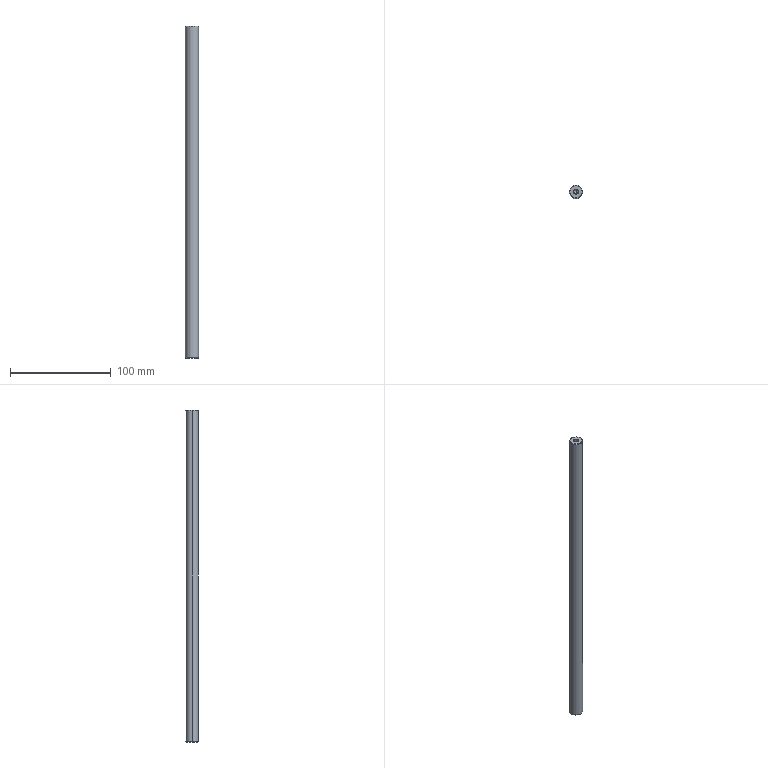Part | STEP file | 001-003-SCD21_D13_L330_M5 | 1 solid | 14 faces | box 13 x 13 x 330 mm | volume 43651 mm3 | cone 8 | cylinder 4 | plane 2 | commonest cylinder face diameters 4.134 x2 13 x2
STEP:
#1=CARTESIAN_POINT('',(0.,0.,0.));
#2=DIRECTION('',(0.,0.,1.));
#3=DIRECTION('',(1.,0.,0.));
#4=AXIS2_PLACEMENT_3D('',#1,#2,#3);
#5=CARTESIAN_POINT('',(0.,2.067,-10.));
#6=VERTEX_POINT('',#5);
#7=CARTESIAN_POINT('',(0.,-2.067,-10.));
#8=VERTEX_POINT('',#7);
#9=CARTESIAN_POINT('',(0.,0.,-10.));
#10=DIRECTION('',(0.,0.,1.));
#11=DIRECTION('',(0.,-1.,0.));
#12=AXIS2_PLACEMENT_3D('',#9,#10,#11);
#13=CIRCLE('',#12,2.067);
#14=CARTESIAN_POINT('',(0.,0.,988.807));
#15=DIRECTION('',(0.,0.,1.));
#16=DIRECTION('',(0.,-1.,0.));
#17=AXIS2_PLACEMENT_3D('',#14,#15,#16);
#18=CONICAL_SURFACE('',#17,1732.051,1.047);
#19=CARTESIAN_POINT('',(0.,-998.807));
#20=DIRECTION('',(1.,0.));
#21=VECTOR('',#20,1.);
#22=LINE('',#19,#21);
#23=(GEOMETRIC_REPRESENTATION_CONTEXT(2)PARAMETRIC_REPRESENTATION_CONTEXT()REPRESENTATION_CONTEXT('',''));
#24=DEFINITIONAL_REPRESENTATION('',(#22),#23);
#25=PCURVE('',#18,#24);
#26=CARTESIAN_POINT('',(0.,0.,-11.193));
#27=DIRECTION('',(0.,0.,1.));
#28=DIRECTION('',(0.,-1.,0.));
#29=AXIS2_PLACEMENT_3D('',#26,#27,#28);
#30=CYLINDRICAL_SURFACE('',#29,2.067);
#31=CARTESIAN_POINT('',(0.,1.193));
#32=DIRECTION('',(1.,0.));
#33=VECTOR('',#32,1.);
#34=LINE('',#31,#33);
#35=(GEOMETRIC_REPRESENTATION_CONTEXT(2)PARAMETRIC_REPRESENTATION_CONTEXT()REPRESENTATION_CONTEXT('',''));
#36=DEFINITIONAL_REPRESENTATION('',(#34),#35);
#37=PCURVE('',#30,#36);
#38=SURFACE_CURVE('',#13,(#25,#37),.PCURVE_S1.);
#39=EDGE_CURVE('',#6,#8,#38,.T.);
#40=ORIENTED_EDGE('',*,*,#39,.F.);
#41=CARTESIAN_POINT('',(0.,0.,-11.193));
#42=VERTEX_POINT('',#41);
#43=CARTESIAN_POINT('',(0.,0.,-11.193));
#44=DIRECTION('',(0.,0.866,0.5));
#45=VECTOR('',#44,1.);
#46=LINE('',#43,#45);
#47=CARTESIAN_POINT('',(3.142,-1000.));
#48=CARTESIAN_POINT('',(3.142,-999.982));
#49=CARTESIAN_POINT('',(3.142,-999.946));
#50=CARTESIAN_POINT('',(3.142,-999.892));
#51=CARTESIAN_POINT('',(3.142,-999.837));
#52=CARTESIAN_POINT('',(3.142,-999.783));
#53=CARTESIAN_POINT('',(3.142,-999.729));
#54=CARTESIAN_POINT('',(3.142,-999.675));
#55=CARTESIAN_POINT('',(3.142,-999.62));
#56=CARTESIAN_POINT('',(3.142,-999.566));
#57=CARTESIAN_POINT('',(3.142,-999.512));
#58=CARTESIAN_POINT('',(3.142,-999.458));
#59=CARTESIAN_POINT('',(3.142,-999.403));
#60=CARTESIAN_POINT('',(3.142,-999.349));
#61=CARTESIAN_POINT('',(3.142,-999.295));
#62=CARTESIAN_POINT('',(3.142,-999.241));
#63=CARTESIAN_POINT('',(3.142,-999.186));
#64=CARTESIAN_POINT('',(3.142,-999.132));
#65=CARTESIAN_POINT('',(3.142,-999.078));
#66=CARTESIAN_POINT('',(3.142,-999.024));
#67=CARTESIAN_POINT('',(3.142,-998.969));
#68=CARTESIAN_POINT('',(3.142,-998.915));
#69=CARTESIAN_POINT('',(3.142,-998.861));
#70=CARTESIAN_POINT('',(3.142,-998.825));
#71=CARTESIAN_POINT('',(3.142,-998.807));
#72=B_SPLINE_CURVE_WITH_KNOTS('',3,(#47,#48,#49,#50,#51,#52,#53,#54,#55,#56,#57,#58,#59,#60,#61,#62,#63,#64,#65,#66,#67,#68,#69,#70,#71),.UNSPECIFIED.,.F.,.F.,(4,1,1,1,1,1,1,1,1,1,1,1,1,1,1,1,1,1,1,1,1,1,4),(0.,0.1085,0.217,0.3255,0.434,0.5424,0.6509,0.7594,0.8679,0.9764,1.085,1.193,1.302,1.41,1.519,1.627,1.736,1.844,1.953,2.061,2.17,2.278,2.387),.QUASI_UNIFORM_KNOTS.);
#73=(GEOMETRIC_REPRESENTATION_CONTEXT(2)PARAMETRIC_REPRESENTATION_CONTEXT()REPRESENTATION_CONTEXT('',''));
#74=DEFINITIONAL_REPRESENTATION('',(#72),#73);
#75=PCURVE('',#18,#74);
#76=CARTESIAN_POINT('',(0.,0.,988.807));
#77=DIRECTION('',(0.,0.,1.));
#78=DIRECTION('',(0.,-1.,0.));
#79=AXIS2_PLACEMENT_3D('',#76,#77,#78);
#80=CONICAL_SURFACE('',#79,1732.051,1.047);
#81=CARTESIAN_POINT('',(3.142,-1000.));
#82=CARTESIAN_POINT('',(3.142,-999.982));
#83=CARTESIAN_POINT('',(3.142,-999.946));
#84=CARTESIAN_POINT('',(3.142,-999.892));
#85=CARTESIAN_POINT('',(3.142,-999.837));
#86=CARTESIAN_POINT('',(3.142,-999.783));
#87=CARTESIAN_POINT('',(3.142,-999.729));
#88=CARTESIAN_POINT('',(3.142,-999.675));
#89=CARTESIAN_POINT('',(3.142,-999.62));
#90=CARTESIAN_POINT('',(3.142,-999.566));
#91=CARTESIAN_POINT('',(3.142,-999.512));
#92=CARTESIAN_POINT('',(3.142,-999.458));
#93=CARTESIAN_POINT('',(3.142,-999.403));
#94=CARTESIAN_POINT('',(3.142,-999.349));
#95=CARTESIAN_POINT('',(3.142,-999.295));
#96=CARTESIAN_POINT('',(3.142,-999.241));
#97=CARTESIAN_POINT('',(3.142,-999.186));
#98=CARTESIAN_POINT('',(3.142,-999.132));
#99=CARTESIAN_POINT('',(3.142,-999.078));
#100=CARTESIAN_POINT('',(3.142,-999.024));
#101=CARTESIAN_POINT('',(3.142,-998.969));
#102=CARTESIAN_POINT('',(3.142,-998.915));
#103=CARTESIAN_POINT('',(3.142,-998.861));
#104=CARTESIAN_POINT('',(3.142,-998.825));
#105=CARTESIAN_POINT('',(3.142,-998.807));
#106=B_SPLINE_CURVE_WITH_KNOTS('',3,(#81,#82,#83,#84,#85,#86,#87,#88,#89,#90,#91,#92,#93,#94,#95,#96,#97,#98,#99,#100,#101,#102,#103,#104,#105),.UNSPECIFIED.,.F.,.F.,(4,1,1,1,1,1,1,1,1,1,1,1,1,1,1,1,1,1,1,1,1,1,4),(0.,0.1085,0.217,0.3255,0.434,0.5424,0.6509,0.7594,0.8679,0.9764,1.085,1.193,1.302,1.41,1.519,1.627,1.736,1.844,1.953,2.061,2.17,2.278,2.387),.QUASI_UNIFORM_KNOTS.);
#107=(GEOMETRIC_REPRESENTATION_CONTEXT(2)PARAMETRIC_REPRESENTATION_CONTEXT()REPRESENTATION_CONTEXT('',''));
#108=DEFINITIONAL_REPRESENTATION('',(#106),#107);
#109=PCURVE('',#80,#108);
#110=SURFACE_CURVE('',#46,(#75,#109),.PCURVE_S1.);
#111=EDGE_CURVE('',#42,#6,#110,.T.);
#112=ORIENTED_EDGE('',*,*,#111,.F.);
#113=CARTESIAN_POINT('',(0.,0.,-11.193));
#114=DIRECTION('',(0.,-0.866,0.5));
#115=VECTOR('',#114,1.);
#116=LINE('',#113,#115);
#117=CARTESIAN_POINT('',(6.283,-1000.));
#118=DIRECTION('',(0.,1.));
#119=VECTOR('',#118,1.);
#120=LINE('',#117,#119);
#121=(GEOMETRIC_REPRESENTATION_CONTEXT(2)PARAMETRIC_REPRESENTATION_CONTEXT()REPRESENTATION_CONTEXT('',''));
#122=DEFINITIONAL_REPRESENTATION('',(#120),#121);
#123=PCURVE('',#18,#122);
#124=CARTESIAN_POINT('',(0.,-1000.));
#125=DIRECTION('',(0.,1.));
#126=VECTOR('',#125,1.);
#127=LINE('',#124,#126);
#128=(GEOMETRIC_REPRESENTATION_CONTEXT(2)PARAMETRIC_REPRESENTATION_CONTEXT()REPRESENTATION_CONTEXT('',''));
#129=DEFINITIONAL_REPRESENTATION('',(#127),#128);
#130=PCURVE('',#80,#129);
#131=SURFACE_CURVE('',#116,(#123,#130),.PCURVE_S1.);
#132=EDGE_CURVE('',#42,#8,#131,.T.);
#133=ORIENTED_EDGE('',*,*,#132,.T.);
#134=EDGE_LOOP('',(#40,#112,#133));
#135=FACE_BOUND('',#134,.F.);
#136=ADVANCED_FACE('',(#135),#18,.F.);
#137=CARTESIAN_POINT('',(0.,-2.067,-0.433));
#138=VERTEX_POINT('',#137);
#139=CARTESIAN_POINT('',(0.,-2.067,-11.193));
#140=DIRECTION('',(0.,0.,1.));
#141=VECTOR('',#140,1.);
#142=LINE('',#139,#141);
#143=CARTESIAN_POINT('',(6.283,0.));
#144=DIRECTION('',(0.,1.));
#145=VECTOR('',#144,1.);
#146=LINE('',#143,#145);
#147=(GEOMETRIC_REPRESENTATION_CONTEXT(2)PARAMETRIC_REPRESENTATION_CONTEXT()REPRESENTATION_CONTEXT('',''));
#148=DEFINITIONAL_REPRESENTATION('',(#146),#147);
#149=PCURVE('',#30,#148);
#150=CARTESIAN_POINT('',(0.,0.,-11.193));
#151=DIRECTION('',(0.,0.,1.));
#152=DIRECTION('',(0.,-1.,0.));
#153=AXIS2_PLACEMENT_3D('',#150,#151,#152);
#154=CYLINDRICAL_SURFACE('',#153,2.067);
#155=CARTESIAN_POINT('',(0.,0.));
#156=DIRECTION('',(0.,1.));
#157=VECTOR('',#156,1.);
#158=LINE('',#155,#157);
#159=(GEOMETRIC_REPRESENTATION_CONTEXT(2)PARAMETRIC_REPRESENTATION_CONTEXT()REPRESENTATION_CONTEXT('',''));
#160=DEFINITIONAL_REPRESENTATION('',(#158),#159);
#161=PCURVE('',#154,#160);
#162=SURFACE_CURVE('',#142,(#149,#161),.PCURVE_S1.);
#163=EDGE_CURVE('',#8,#138,#162,.T.);
#164=ORIENTED_EDGE('',*,*,#163,.T.);
#165=CARTESIAN_POINT('',(0.,2.067,-0.433));
#166=VERTEX_POINT('',#165);
#167=CARTESIAN_POINT('',(0.,0.,-0.433));
#168=DIRECTION('',(0.,0.,1.));
#169=DIRECTION('',(0.,-1.,0.));
#170=AXIS2_PLACEMENT_3D('',#167,#168,#169);
#171=CIRCLE('',#170,2.067);
#172=CARTESIAN_POINT('',(0.,10.76));
#173=DIRECTION('',(1.,0.));
#174=VECTOR('',#173,1.);
#175=LINE('',#172,#174);
#176=(GEOMETRIC_REPRESENTATION_CONTEXT(2)PARAMETRIC_REPRESENTATION_CONTEXT()REPRESENTATION_CONTEXT('',''));
#177=DEFINITIONAL_REPRESENTATION('',(#175),#176);
#178=PCURVE('',#30,#177);
#179=CARTESIAN_POINT('',(0.,0.,-0.433));
#180=DIRECTION('',(0.,0.,1.));
#181=DIRECTION('',(0.,-1.,0.));
#182=AXIS2_PLACEMENT_3D('',#179,#180,#181);
#183=CONICAL_SURFACE('',#182,2.067,0.7854);
#184=CARTESIAN_POINT('',(0.,0.));
#185=DIRECTION('',(1.,0.));
#186=VECTOR('',#185,1.);
#187=LINE('',#184,#186);
#188=(GEOMETRIC_REPRESENTATION_CONTEXT(2)PARAMETRIC_REPRESENTATION_CONTEXT()REPRESENTATION_CONTEXT('',''));
#189=DEFINITIONAL_REPRESENTATION('',(#187),#188);
#190=PCURVE('',#183,#189);
#191=SURFACE_CURVE('',#171,(#178,#190),.PCURVE_S1.);
#192=EDGE_CURVE('',#166,#138,#191,.T.);
#193=ORIENTED_EDGE('',*,*,#192,.F.);
#194=CARTESIAN_POINT('',(0.,2.067,-11.193));
#195=DIRECTION('',(0.,0.,1.));
#196=VECTOR('',#195,1.);
#197=LINE('',#194,#196);
#198=CARTESIAN_POINT('',(3.142,0.));
#199=DIRECTION('',(0.,1.));
#200=VECTOR('',#199,1.);
#201=LINE('',#198,#200);
#202=(GEOMETRIC_REPRESENTATION_CONTEXT(2)PARAMETRIC_REPRESENTATION_CONTEXT()REPRESENTATION_CONTEXT('',''));
#203=DEFINITIONAL_REPRESENTATION('',(#201),#202);
#204=PCURVE('',#30,#203);
#205=CARTESIAN_POINT('',(3.142,0.));
#206=DIRECTION('',(0.,1.));
#207=VECTOR('',#206,1.);
#208=LINE('',#205,#207);
#209=(GEOMETRIC_REPRESENTATION_CONTEXT(2)PARAMETRIC_REPRESENTATION_CONTEXT()REPRESENTATION_CONTEXT('',''));
#210=DEFINITIONAL_REPRESENTATION('',(#208),#209);
#211=PCURVE('',#154,#210);
#212=SURFACE_CURVE('',#197,(#204,#211),.PCURVE_S1.);
#213=EDGE_CURVE('',#6,#166,#212,.T.);
#214=ORIENTED_EDGE('',*,*,#213,.F.);
#215=ORIENTED_EDGE('',*,*,#39,.T.);
#216=EDGE_LOOP('',(#164,#193,#214,#215));
#217=FACE_BOUND('',#216,.F.);
#218=ADVANCED_FACE('',(#217),#30,.F.);
#219=CARTESIAN_POINT('',(0.,-2.5,0.));
#220=VERTEX_POINT('',#219);
#221=CARTESIAN_POINT('',(0.,-2.067,-0.433));
#222=DIRECTION('',(0.,-0.7071,0.7071));
#223=VECTOR('',#222,1.);
#224=LINE('',#221,#223);
#225=CARTESIAN_POINT('',(6.283,0.));
#226=DIRECTION('',(0.,1.));
#227=VECTOR('',#226,1.);
#228=LINE('',#225,#227);
#229=(GEOMETRIC_REPRESENTATION_CONTEXT(2)PARAMETRIC_REPRESENTATION_CONTEXT()REPRESENTATION_CONTEXT('',''));
#230=DEFINITIONAL_REPRESENTATION('',(#228),#229);
#231=PCURVE('',#183,#230);
#232=CARTESIAN_POINT('',(0.,0.,-0.433));
#233=DIRECTION('',(0.,0.,1.));
#234=DIRECTION('',(0.,-1.,0.));
#235=AXIS2_PLACEMENT_3D('',#232,#233,#234);
#236=CONICAL_SURFACE('',#235,2.067,0.7854);
#237=CARTESIAN_POINT('',(0.,0.));
#238=DIRECTION('',(0.,1.));
#239=VECTOR('',#238,1.);
#240=LINE('',#237,#239);
#241=(GEOMETRIC_REPRESENTATION_CONTEXT(2)PARAMETRIC_REPRESENTATION_CONTEXT()REPRESENTATION_CONTEXT('',''));
#242=DEFINITIONAL_REPRESENTATION('',(#240),#241);
#243=PCURVE('',#236,#242);
#244=SURFACE_CURVE('',#224,(#231,#243),.PCURVE_S1.);
#245=EDGE_CURVE('',#138,#220,#244,.T.);
#246=ORIENTED_EDGE('',*,*,#245,.T.);
#247=CARTESIAN_POINT('',(0.,2.5,0.));
#248=VERTEX_POINT('',#247);
#249=CARTESIAN_POINT('',(0.,0.,0.));
#250=DIRECTION('',(0.,0.,1.));
#251=DIRECTION('',(0.,-1.,0.));
#252=AXIS2_PLACEMENT_3D('',#249,#250,#251);
#253=CIRCLE('',#252,2.5);
#254=CARTESIAN_POINT('',(0.,0.433));
#255=DIRECTION('',(1.,0.));
#256=VECTOR('',#255,1.);
#257=LINE('',#254,#256);
#258=(GEOMETRIC_REPRESENTATION_CONTEXT(2)PARAMETRIC_REPRESENTATION_CONTEXT()REPRESENTATION_CONTEXT('',''));
#259=DEFINITIONAL_REPRESENTATION('',(#257),#258);
#260=PCURVE('',#183,#259);
#261=CARTESIAN_POINT('',(0.,0.,0.));
#262=DIRECTION('',(0.,0.,-1.));
#263=DIRECTION('',(-1.,0.,0.));
#264=AXIS2_PLACEMENT_3D('',#261,#262,#263);
#265=PLANE('',#264);
#266=CARTESIAN_POINT('',(0.,-2.5));
#267=CARTESIAN_POINT('',(-4.33,-2.5));
#268=CARTESIAN_POINT('',(-2.165,1.25));
#269=CARTESIAN_POINT('',(0.,5.));
#270=CARTESIAN_POINT('',(2.165,1.25));
#271=CARTESIAN_POINT('',(4.33,-2.5));
#272=CARTESIAN_POINT('',(0.,-2.5));
#273=(BOUNDED_CURVE()B_SPLINE_CURVE(2,(#266,#267,#268,#269,#270,#271,#272),.UNSPECIFIED.,.T.,.F.)B_SPLINE_CURVE_WITH_KNOTS((1,2,2,2,2,1),(-2.094,0.,2.094,4.189,6.283,8.378),.UNSPECIFIED.)CURVE()GEOMETRIC_REPRESENTATION_ITEM()RATIONAL_B_SPLINE_CURVE((1.,0.5,1.,0.5,1.,0.5,1.))REPRESENTATION_ITEM(''));
#274=(GEOMETRIC_REPRESENTATION_CONTEXT(2)PARAMETRIC_REPRESENTATION_CONTEXT()REPRESENTATION_CONTEXT('',''));
#275=DEFINITIONAL_REPRESENTATION('',(#273),#274);
#276=PCURVE('',#265,#275);
#277=SURFACE_CURVE('',#253,(#260,#276),.PCURVE_S1.);
#278=EDGE_CURVE('',#248,#220,#277,.T.);
#279=ORIENTED_EDGE('',*,*,#278,.F.);
#280=CARTESIAN_POINT('',(0.,2.067,-0.433));
#281=DIRECTION('',(0.,0.7071,0.7071));
#282=VECTOR('',#281,1.);
#283=LINE('',#280,#282);
#284=CARTESIAN_POINT('',(3.142,0.));
#285=DIRECTION('',(0.,1.));
#286=VECTOR('',#285,1.);
#287=LINE('',#284,#286);
#288=(GEOMETRIC_REPRESENTATION_CONTEXT(2)PARAMETRIC_REPRESENTATION_CONTEXT()REPRESENTATION_CONTEXT('',''));
#289=DEFINITIONAL_REPRESENTATION('',(#287),#288);
#290=PCURVE('',#183,#289);
#291=CARTESIAN_POINT('',(3.142,0.));
#292=DIRECTION('',(0.,1.));
#293=VECTOR('',#292,1.);
#294=LINE('',#291,#293);
#295=(GEOMETRIC_REPRESENTATION_CONTEXT(2)PARAMETRIC_REPRESENTATION_CONTEXT()REPRESENTATION_CONTEXT('',''));
#296=DEFINITIONAL_REPRESENTATION('',(#294),#295);
#297=PCURVE('',#236,#296);
#298=SURFACE_CURVE('',#283,(#290,#297),.PCURVE_S1.);
#299=EDGE_CURVE('',#166,#248,#298,.T.);
#300=ORIENTED_EDGE('',*,*,#299,.F.);
#301=ORIENTED_EDGE('',*,*,#192,.T.);
#302=EDGE_LOOP('',(#246,#279,#300,#301));
#303=FACE_BOUND('',#302,.F.);
#304=ADVANCED_FACE('',(#303),#183,.F.);
#305=CARTESIAN_POINT('',(6.,0.,-330.));
#306=VERTEX_POINT('',#305);
#307=CARTESIAN_POINT('',(-6.,0.,-330.));
#308=VERTEX_POINT('',#307);
#309=CARTESIAN_POINT('',(0.,0.,-330.));
#310=DIRECTION('',(0.,0.,1.));
#311=DIRECTION('',(1.,0.,0.));
#312=AXIS2_PLACEMENT_3D('',#309,#310,#311);
#313=CIRCLE('',#312,6.);
#314=CARTESIAN_POINT('',(0.,0.,-330.));
#315=DIRECTION('',(0.,0.,1.));
#316=DIRECTION('',(1.,0.,0.));
#317=AXIS2_PLACEMENT_3D('',#314,#315,#316);
#318=CONICAL_SURFACE('',#317,6.,0.7854);
#319=CARTESIAN_POINT('',(0.,0.));
#320=DIRECTION('',(1.,0.));
#321=VECTOR('',#320,1.);
#322=LINE('',#319,#321);
#323=(GEOMETRIC_REPRESENTATION_CONTEXT(2)PARAMETRIC_REPRESENTATION_CONTEXT()REPRESENTATION_CONTEXT('',''));
#324=DEFINITIONAL_REPRESENTATION('',(#322),#323);
#325=PCURVE('',#318,#324);
#326=CARTESIAN_POINT('',(0.,6.,-330.));
#327=DIRECTION('',(0.,0.,1.));
#328=DIRECTION('',(1.,0.,0.));
#329=AXIS2_PLACEMENT_3D('',#326,#327,#328);
#330=PLANE('',#329);
#331=CARTESIAN_POINT('',(0.,-6.));
#332=DIRECTION('',(1.,0.));
#333=AXIS2_PLACEMENT_2D('',#331,#332);
#334=CIRCLE('',#333,6.);
#335=(GEOMETRIC_REPRESENTATION_CONTEXT(2)PARAMETRIC_REPRESENTATION_CONTEXT()REPRESENTATION_CONTEXT('',''));
#336=DEFINITIONAL_REPRESENTATION('',(#334),#335);
#337=PCURVE('',#330,#336);
#338=SURFACE_CURVE('',#313,(#325,#337),.PCURVE_S1.);
#339=EDGE_CURVE('',#306,#308,#338,.T.);
#340=ORIENTED_EDGE('',*,*,#339,.T.);
#341=CARTESIAN_POINT('',(-6.5,0.,-329.5));
#342=VERTEX_POINT('',#341);
#343=CARTESIAN_POINT('',(-6.,0.,-330.));
#344=DIRECTION('',(-0.7071,0.,0.7071));
#345=VECTOR('',#344,1.);
#346=LINE('',#343,#345);
#347=CARTESIAN_POINT('',(3.142,0.));
#348=DIRECTION('',(0.,1.));
#349=VECTOR('',#348,1.);
#350=LINE('',#347,#349);
#351=(GEOMETRIC_REPRESENTATION_CONTEXT(2)PARAMETRIC_REPRESENTATION_CONTEXT()REPRESENTATION_CONTEXT('',''));
#352=DEFINITIONAL_REPRESENTATION('',(#350),#351);
#353=PCURVE('',#318,#352);
#354=CARTESIAN_POINT('',(0.,0.,-330.));
#355=DIRECTION('',(0.,0.,1.));
#356=DIRECTION('',(1.,0.,0.));
#357=AXIS2_PLACEMENT_3D('',#354,#355,#356);
#358=CONICAL_SURFACE('',#357,6.,0.7854);
#359=CARTESIAN_POINT('',(3.142,0.));
#360=DIRECTION('',(0.,1.));
#361=VECTOR('',#360,1.);
#362=LINE('',#359,#361);
#363=(GEOMETRIC_REPRESENTATION_CONTEXT(2)PARAMETRIC_REPRESENTATION_CONTEXT()REPRESENTATION_CONTEXT('',''));
#364=DEFINITIONAL_REPRESENTATION('',(#362),#363);
#365=PCURVE('',#358,#364);
#366=SURFACE_CURVE('',#346,(#353,#365),.PCURVE_S1.);
#367=EDGE_CURVE('',#308,#342,#366,.T.);
#368=ORIENTED_EDGE('',*,*,#367,.T.);
#369=CARTESIAN_POINT('',(6.5,0.,-329.5));
#370=VERTEX_POINT('',#369);
#371=CARTESIAN_POINT('',(0.,0.,-329.5));
#372=DIRECTION('',(0.,0.,1.));
#373=DIRECTION('',(1.,0.,0.));
#374=AXIS2_PLACEMENT_3D('',#371,#372,#373);
#375=CIRCLE('',#374,6.5);
#376=CARTESIAN_POINT('',(0.,0.5));
#377=DIRECTION('',(1.,0.));
#378=VECTOR('',#377,1.);
#379=LINE('',#376,#378);
#380=(GEOMETRIC_REPRESENTATION_CONTEXT(2)PARAMETRIC_REPRESENTATION_CONTEXT()REPRESENTATION_CONTEXT('',''));
#381=DEFINITIONAL_REPRESENTATION('',(#379),#380);
#382=PCURVE('',#318,#381);
#383=CARTESIAN_POINT('',(0.,0.,-330.));
#384=DIRECTION('',(0.,0.,1.));
#385=DIRECTION('',(1.,0.,0.));
#386=AXIS2_PLACEMENT_3D('',#383,#384,#385);
#387=CYLINDRICAL_SURFACE('',#386,6.5);
#388=CARTESIAN_POINT('',(0.,0.5));
#389=DIRECTION('',(1.,0.));
#390=VECTOR('',#389,1.);
#391=LINE('',#388,#390);
#392=(GEOMETRIC_REPRESENTATION_CONTEXT(2)PARAMETRIC_REPRESENTATION_CONTEXT()REPRESENTATION_CONTEXT('',''));
#393=DEFINITIONAL_REPRESENTATION('',(#391),#392);
#394=PCURVE('',#387,#393);
#395=SURFACE_CURVE('',#375,(#382,#394),.PCURVE_S1.);
#396=EDGE_CURVE('',#370,#342,#395,.T.);
#397=ORIENTED_EDGE('',*,*,#396,.F.);
#398=CARTESIAN_POINT('',(6.,0.,-330.));
#399=DIRECTION('',(0.7071,0.,0.7071));
#400=VECTOR('',#399,1.);
#401=LINE('',#398,#400);
#402=CARTESIAN_POINT('',(0.,0.));
#403=DIRECTION('',(0.,1.));
#404=VECTOR('',#403,1.);
#405=LINE('',#402,#404);
#406=(GEOMETRIC_REPRESENTATION_CONTEXT(2)PARAMETRIC_REPRESENTATION_CONTEXT()REPRESENTATION_CONTEXT('',''));
#407=DEFINITIONAL_REPRESENTATION('',(#405),#406);
#408=PCURVE('',#318,#407);
#409=CARTESIAN_POINT('',(6.283,0.));
#410=DIRECTION('',(0.,1.));
#411=VECTOR('',#410,1.);
#412=LINE('',#409,#411);
#413=(GEOMETRIC_REPRESENTATION_CONTEXT(2)PARAMETRIC_REPRESENTATION_CONTEXT()REPRESENTATION_CONTEXT('',''));
#414=DEFINITIONAL_REPRESENTATION('',(#412),#413);
#415=PCURVE('',#358,#414);
#416=SURFACE_CURVE('',#401,(#408,#415),.PCURVE_S1.);
#417=EDGE_CURVE('',#306,#370,#416,.T.);
#418=ORIENTED_EDGE('',*,*,#417,.F.);
#419=EDGE_LOOP('',(#340,#368,#397,#418));
#420=FACE_BOUND('',#419,.T.);
#421=ADVANCED_FACE('',(#420),#318,.T.);
#422=ORIENTED_EDGE('',*,*,#396,.T.);
#423=CARTESIAN_POINT('',(-6.5,0.,-0.5));
#424=VERTEX_POINT('',#423);
#425=CARTESIAN_POINT('',(-6.5,0.,-330.));
#426=DIRECTION('',(0.,0.,1.));
#427=VECTOR('',#426,1.);
#428=LINE('',#425,#427);
#429=CARTESIAN_POINT('',(3.142,0.));
#430=DIRECTION('',(0.,1.));
#431=VECTOR('',#430,1.);
#432=LINE('',#429,#431);
#433=(GEOMETRIC_REPRESENTATION_CONTEXT(2)PARAMETRIC_REPRESENTATION_CONTEXT()REPRESENTATION_CONTEXT('',''));
#434=DEFINITIONAL_REPRESENTATION('',(#432),#433);
#435=PCURVE('',#387,#434);
#436=CARTESIAN_POINT('',(0.,0.,-330.));
#437=DIRECTION('',(0.,0.,1.));
#438=DIRECTION('',(1.,0.,0.));
#439=AXIS2_PLACEMENT_3D('',#436,#437,#438);
#440=CYLINDRICAL_SURFACE('',#439,6.5);
#441=CARTESIAN_POINT('',(3.142,0.));
#442=DIRECTION('',(0.,1.));
#443=VECTOR('',#442,1.);
#444=LINE('',#441,#443);
#445=(GEOMETRIC_REPRESENTATION_CONTEXT(2)PARAMETRIC_REPRESENTATION_CONTEXT()REPRESENTATION_CONTEXT('',''));
#446=DEFINITIONAL_REPRESENTATION('',(#444),#445);
#447=PCURVE('',#440,#446);
#448=SURFACE_CURVE('',#428,(#435,#447),.PCURVE_S1.);
#449=EDGE_CURVE('',#342,#424,#448,.T.);
#450=ORIENTED_EDGE('',*,*,#449,.T.);
#451=CARTESIAN_POINT('',(6.5,0.,-0.5));
#452=VERTEX_POINT('',#451);
#453=CARTESIAN_POINT('',(0.,0.,-0.5));
#454=DIRECTION('',(0.,0.,1.));
#455=DIRECTION('',(1.,0.,0.));
#456=AXIS2_PLACEMENT_3D('',#453,#454,#455);
#457=CIRCLE('',#456,6.5);
#458=CARTESIAN_POINT('',(0.,329.5));
#459=DIRECTION('',(1.,0.));
#460=VECTOR('',#459,1.);
#461=LINE('',#458,#460);
#462=(GEOMETRIC_REPRESENTATION_CONTEXT(2)PARAMETRIC_REPRESENTATION_CONTEXT()REPRESENTATION_CONTEXT('',''));
#463=DEFINITIONAL_REPRESENTATION('',(#461),#462);
#464=PCURVE('',#387,#463);
#465=CARTESIAN_POINT('',(0.,0.,-0.5));
#466=DIRECTION('',(0.,0.,-1.));
#467=DIRECTION('',(-1.,0.,0.));
#468=AXIS2_PLACEMENT_3D('',#465,#466,#467);
#469=CONICAL_SURFACE('',#468,6.5,0.7854);
#470=CARTESIAN_POINT('',(3.142,0.));
#471=DIRECTION('',(-1.,0.));
#472=VECTOR('',#471,1.);
#473=LINE('',#470,#472);
#474=(GEOMETRIC_REPRESENTATION_CONTEXT(2)PARAMETRIC_REPRESENTATION_CONTEXT()REPRESENTATION_CONTEXT('',''));
#475=DEFINITIONAL_REPRESENTATION('',(#473),#474);
#476=PCURVE('',#469,#475);
#477=SURFACE_CURVE('',#457,(#464,#476),.PCURVE_S1.);
#478=EDGE_CURVE('',#452,#424,#477,.T.);
#479=ORIENTED_EDGE('',*,*,#478,.F.);
#480=CARTESIAN_POINT('',(6.5,0.,-330.));
#481=DIRECTION('',(0.,0.,1.));
#482=VECTOR('',#481,1.);
#483=LINE('',#480,#482);
#484=CARTESIAN_POINT('',(0.,0.));
#485=DIRECTION('',(0.,1.));
#486=VECTOR('',#485,1.);
#487=LINE('',#484,#486);
#488=(GEOMETRIC_REPRESENTATION_CONTEXT(2)PARAMETRIC_REPRESENTATION_CONTEXT()REPRESENTATION_CONTEXT('',''));
#489=DEFINITIONAL_REPRESENTATION('',(#487),#488);
#490=PCURVE('',#387,#489);
#491=CARTESIAN_POINT('',(6.283,0.));
#492=DIRECTION('',(0.,1.));
#493=VECTOR('',#492,1.);
#494=LINE('',#491,#493);
#495=(GEOMETRIC_REPRESENTATION_CONTEXT(2)PARAMETRIC_REPRESENTATION_CONTEXT()REPRESENTATION_CONTEXT('',''));
#496=DEFINITIONAL_REPRESENTATION('',(#494),#495);
#497=PCURVE('',#440,#496);
#498=SURFACE_CURVE('',#483,(#490,#497),.PCURVE_S1.);
#499=EDGE_CURVE('',#370,#452,#498,.T.);
#500=ORIENTED_EDGE('',*,*,#499,.F.);
#501=EDGE_LOOP('',(#422,#450,#479,#500));
#502=FACE_BOUND('',#501,.T.);
#503=ADVANCED_FACE('',(#502),#387,.T.);
#504=CARTESIAN_POINT('',(6.,0.,0.));
#505=VERTEX_POINT('',#504);
#506=CARTESIAN_POINT('',(-6.,0.,0.));
#507=VERTEX_POINT('',#506);
#508=CARTESIAN_POINT('',(0.,0.,0.));
#509=DIRECTION('',(0.,0.,1.));
#510=DIRECTION('',(1.,0.,0.));
#511=AXIS2_PLACEMENT_3D('',#508,#509,#510);
#512=CIRCLE('',#511,6.);
#513=CARTESIAN_POINT('',(3.142,-0.5));
#514=DIRECTION('',(-1.,0.));
#515=VECTOR('',#514,1.);
#516=LINE('',#513,#515);
#517=(GEOMETRIC_REPRESENTATION_CONTEXT(2)PARAMETRIC_REPRESENTATION_CONTEXT()REPRESENTATION_CONTEXT('',''));
#518=DEFINITIONAL_REPRESENTATION('',(#516),#517);
#519=PCURVE('',#469,#518);
#520=CARTESIAN_POINT('',(-6.,0.));
#521=CARTESIAN_POINT('',(-6.,10.392));
#522=CARTESIAN_POINT('',(3.,5.196));
#523=CARTESIAN_POINT('',(12.,0.));
#524=CARTESIAN_POINT('',(3.,-5.196));
#525=CARTESIAN_POINT('',(-6.,-10.392));
#526=CARTESIAN_POINT('',(-6.,0.));
#527=(BOUNDED_CURVE()B_SPLINE_CURVE(2,(#520,#521,#522,#523,#524,#525,#526),.UNSPECIFIED.,.T.,.F.)B_SPLINE_CURVE_WITH_KNOTS((1,2,2,2,2,1),(-2.094,0.,2.094,4.189,6.283,8.378),.UNSPECIFIED.)CURVE()GEOMETRIC_REPRESENTATION_ITEM()RATIONAL_B_SPLINE_CURVE((1.,0.5,1.,0.5,1.,0.5,1.))REPRESENTATION_ITEM(''));
#528=(GEOMETRIC_REPRESENTATION_CONTEXT(2)PARAMETRIC_REPRESENTATION_CONTEXT()REPRESENTATION_CONTEXT('',''));
#529=DEFINITIONAL_REPRESENTATION('',(#527),#528);
#530=PCURVE('',#265,#529);
#531=SURFACE_CURVE('',#512,(#519,#530),.PCURVE_S1.);
#532=EDGE_CURVE('',#505,#507,#531,.T.);
#533=ORIENTED_EDGE('',*,*,#532,.F.);
#534=CARTESIAN_POINT('',(6.5,0.,-0.5));
#535=DIRECTION('',(0.7071,0.,-0.7071));
#536=VECTOR('',#535,1.);
#537=LINE('',#534,#536);
#538=CARTESIAN_POINT('',(3.142,0.));
#539=DIRECTION('',(0.,1.));
#540=VECTOR('',#539,1.);
#541=LINE('',#538,#540);
#542=(GEOMETRIC_REPRESENTATION_CONTEXT(2)PARAMETRIC_REPRESENTATION_CONTEXT()REPRESENTATION_CONTEXT('',''));
#543=DEFINITIONAL_REPRESENTATION('',(#541),#542);
#544=PCURVE('',#469,#543);
#545=CARTESIAN_POINT('',(0.,0.,-0.5));
#546=DIRECTION('',(0.,0.,-1.));
#547=DIRECTION('',(-1.,0.,0.));
#548=AXIS2_PLACEMENT_3D('',#545,#546,#547);
#549=CONICAL_SURFACE('',#548,6.5,0.7854);
#550=CARTESIAN_POINT('',(3.142,0.));
#551=DIRECTION('',(0.,1.));
#552=VECTOR('',#551,1.);
#553=LINE('',#550,#552);
#554=(GEOMETRIC_REPRESENTATION_CONTEXT(2)PARAMETRIC_REPRESENTATION_CONTEXT()REPRESENTATION_CONTEXT('',''));
#555=DEFINITIONAL_REPRESENTATION('',(#553),#554);
#556=PCURVE('',#549,#555);
#557=SURFACE_CURVE('',#537,(#544,#556),.PCURVE_S1.);
#558=EDGE_CURVE('',#505,#452,#557,.T.);
#559=ORIENTED_EDGE('',*,*,#558,.T.);
#560=ORIENTED_EDGE('',*,*,#478,.T.);
#561=CARTESIAN_POINT('',(-6.5,0.,-0.5));
#562=DIRECTION('',(-0.7071,0.,-0.7071));
#563=VECTOR('',#562,1.);
#564=LINE('',#561,#563);
#565=CARTESIAN_POINT('',(0.,0.));
#566=DIRECTION('',(0.,1.));
#567=VECTOR('',#566,1.);
#568=LINE('',#565,#567);
#569=(GEOMETRIC_REPRESENTATION_CONTEXT(2)PARAMETRIC_REPRESENTATION_CONTEXT()REPRESENTATION_CONTEXT('',''));
#570=DEFINITIONAL_REPRESENTATION('',(#568),#569);
#571=PCURVE('',#469,#570);
#572=CARTESIAN_POINT('',(6.283,0.));
#573=DIRECTION('',(0.,1.));
#574=VECTOR('',#573,1.);
#575=LINE('',#572,#574);
#576=(GEOMETRIC_REPRESENTATION_CONTEXT(2)PARAMETRIC_REPRESENTATION_CONTEXT()REPRESENTATION_CONTEXT('',''));
#577=DEFINITIONAL_REPRESENTATION('',(#575),#576);
#578=PCURVE('',#549,#577);
#579=SURFACE_CURVE('',#564,(#571,#578),.PCURVE_S1.);
#580=EDGE_CURVE('',#507,#424,#579,.T.);
#581=ORIENTED_EDGE('',*,*,#580,.F.);
#582=EDGE_LOOP('',(#533,#559,#560,#581));
#583=FACE_BOUND('',#582,.T.);
#584=ADVANCED_FACE('',(#583),#469,.T.);
#585=CARTESIAN_POINT('',(0.,0.,0.));
#586=DIRECTION('',(0.,0.,1.));
#587=DIRECTION('',(0.,-1.,0.));
#588=AXIS2_PLACEMENT_3D('',#585,#586,#587);
#589=CIRCLE('',#588,2.5);
#590=CARTESIAN_POINT('',(0.,-2.5));
#591=CARTESIAN_POINT('',(-4.33,-2.5));
#592=CARTESIAN_POINT('',(-2.165,1.25));
#593=CARTESIAN_POINT('',(0.,5.));
#594=CARTESIAN_POINT('',(2.165,1.25));
#595=CARTESIAN_POINT('',(4.33,-2.5));
#596=CARTESIAN_POINT('',(0.,-2.5));
#597=(BOUNDED_CURVE()B_SPLINE_CURVE(2,(#590,#591,#592,#593,#594,#595,#596),.UNSPECIFIED.,.T.,.F.)B_SPLINE_CURVE_WITH_KNOTS((1,2,2,2,2,1),(-2.094,0.,2.094,4.189,6.283,8.378),.UNSPECIFIED.)CURVE()GEOMETRIC_REPRESENTATION_ITEM()RATIONAL_B_SPLINE_CURVE((1.,0.5,1.,0.5,1.,0.5,1.))REPRESENTATION_ITEM(''));
#598=(GEOMETRIC_REPRESENTATION_CONTEXT(2)PARAMETRIC_REPRESENTATION_CONTEXT()REPRESENTATION_CONTEXT('',''));
#599=DEFINITIONAL_REPRESENTATION('',(#597),#598);
#600=PCURVE('',#265,#599);
#601=CARTESIAN_POINT('',(0.,0.433));
#602=DIRECTION('',(1.,0.));
#603=VECTOR('',#602,1.);
#604=LINE('',#601,#603);
#605=(GEOMETRIC_REPRESENTATION_CONTEXT(2)PARAMETRIC_REPRESENTATION_CONTEXT()REPRESENTATION_CONTEXT('',''));
#606=DEFINITIONAL_REPRESENTATION('',(#604),#605);
#607=PCURVE('',#236,#606);
#608=SURFACE_CURVE('',#589,(#600,#607),.PCURVE_S1.);
#609=EDGE_CURVE('',#220,#248,#608,.T.);
#610=ORIENTED_EDGE('',*,*,#609,.F.);
#611=ORIENTED_EDGE('',*,*,#278,.F.);
#612=EDGE_LOOP('',(#610,#611));
#613=FACE_BOUND('',#612,.T.);
#614=CARTESIAN_POINT('',(0.,0.,0.));
#615=DIRECTION('',(0.,0.,1.));
#616=DIRECTION('',(1.,0.,0.));
#617=AXIS2_PLACEMENT_3D('',#614,#615,#616);
#618=CIRCLE('',#617,6.);
#619=CARTESIAN_POINT('',(-6.,0.));
#620=CARTESIAN_POINT('',(-6.,10.392));
#621=CARTESIAN_POINT('',(3.,5.196));
#622=CARTESIAN_POINT('',(12.,0.));
#623=CARTESIAN_POINT('',(3.,-5.196));
#624=CARTESIAN_POINT('',(-6.,-10.392));
#625=CARTESIAN_POINT('',(-6.,0.));
#626=(BOUNDED_CURVE()B_SPLINE_CURVE(2,(#619,#620,#621,#622,#623,#624,#625),.UNSPECIFIED.,.T.,.F.)B_SPLINE_CURVE_WITH_KNOTS((1,2,2,2,2,1),(-2.094,0.,2.094,4.189,6.283,8.378),.UNSPECIFIED.)CURVE()GEOMETRIC_REPRESENTATION_ITEM()RATIONAL_B_SPLINE_CURVE((1.,0.5,1.,0.5,1.,0.5,1.))REPRESENTATION_ITEM(''));
#627=(GEOMETRIC_REPRESENTATION_CONTEXT(2)PARAMETRIC_REPRESENTATION_CONTEXT()REPRESENTATION_CONTEXT('',''));
#628=DEFINITIONAL_REPRESENTATION('',(#626),#627);
#629=PCURVE('',#265,#628);
#630=CARTESIAN_POINT('',(9.425,-0.5));
#631=DIRECTION('',(-1.,0.));
#632=VECTOR('',#631,1.);
#633=LINE('',#630,#632);
#634=(GEOMETRIC_REPRESENTATION_CONTEXT(2)PARAMETRIC_REPRESENTATION_CONTEXT()REPRESENTATION_CONTEXT('',''));
#635=DEFINITIONAL_REPRESENTATION('',(#633),#634);
#636=PCURVE('',#549,#635);
#637=SURFACE_CURVE('',#618,(#629,#636),.PCURVE_S1.);
#638=EDGE_CURVE('',#507,#505,#637,.T.);
#639=ORIENTED_EDGE('',*,*,#638,.T.);
#640=ORIENTED_EDGE('',*,*,#532,.T.);
#641=EDGE_LOOP('',(#639,#640));
#642=FACE_BOUND('',#641,.T.);
#643=ADVANCED_FACE('',(#613,#642),#265,.F.);
#644=ORIENTED_EDGE('',*,*,#558,.F.);
#645=ORIENTED_EDGE('',*,*,#638,.F.);
#646=ORIENTED_EDGE('',*,*,#580,.T.);
#647=CARTESIAN_POINT('',(0.,0.,-0.5));
#648=DIRECTION('',(0.,0.,1.));
#649=DIRECTION('',(1.,0.,0.));
#650=AXIS2_PLACEMENT_3D('',#647,#648,#649);
#651=CIRCLE('',#650,6.5);
#652=CARTESIAN_POINT('',(9.425,0.));
#653=DIRECTION('',(-1.,0.));
#654=VECTOR('',#653,1.);
#655=LINE('',#652,#654);
#656=(GEOMETRIC_REPRESENTATION_CONTEXT(2)PARAMETRIC_REPRESENTATION_CONTEXT()REPRESENTATION_CONTEXT('',''));
#657=DEFINITIONAL_REPRESENTATION('',(#655),#656);
#658=PCURVE('',#549,#657);
#659=CARTESIAN_POINT('',(0.,329.5));
#660=DIRECTION('',(1.,0.));
#661=VECTOR('',#660,1.);
#662=LINE('',#659,#661);
#663=(GEOMETRIC_REPRESENTATION_CONTEXT(2)PARAMETRIC_REPRESENTATION_CONTEXT()REPRESENTATION_CONTEXT('',''));
#664=DEFINITIONAL_REPRESENTATION('',(#662),#663);
#665=PCURVE('',#440,#664);
#666=SURFACE_CURVE('',#651,(#658,#665),.PCURVE_S1.);
#667=EDGE_CURVE('',#424,#452,#666,.T.);
#668=ORIENTED_EDGE('',*,*,#667,.T.);
#669=EDGE_LOOP('',(#644,#645,#646,#668));
#670=FACE_BOUND('',#669,.T.);
#671=ADVANCED_FACE('',(#670),#549,.T.);
#672=ORIENTED_EDGE('',*,*,#449,.F.);
#673=CARTESIAN_POINT('',(0.,0.,-329.5));
#674=DIRECTION('',(0.,0.,1.));
#675=DIRECTION('',(1.,0.,0.));
#676=AXIS2_PLACEMENT_3D('',#673,#674,#675);
#677=CIRCLE('',#676,6.5);
#678=CARTESIAN_POINT('',(0.,0.5));
#679=DIRECTION('',(1.,0.));
#680=VECTOR('',#679,1.);
#681=LINE('',#678,#680);
#682=(GEOMETRIC_REPRESENTATION_CONTEXT(2)PARAMETRIC_REPRESENTATION_CONTEXT()REPRESENTATION_CONTEXT('',''));
#683=DEFINITIONAL_REPRESENTATION('',(#681),#682);
#684=PCURVE('',#440,#683);
#685=CARTESIAN_POINT('',(0.,0.5));
#686=DIRECTION('',(1.,0.));
#687=VECTOR('',#686,1.);
#688=LINE('',#685,#687);
#689=(GEOMETRIC_REPRESENTATION_CONTEXT(2)PARAMETRIC_REPRESENTATION_CONTEXT()REPRESENTATION_CONTEXT('',''));
#690=DEFINITIONAL_REPRESENTATION('',(#688),#689);
#691=PCURVE('',#358,#690);
#692=SURFACE_CURVE('',#677,(#684,#691),.PCURVE_S1.);
#693=EDGE_CURVE('',#342,#370,#692,.T.);
#694=ORIENTED_EDGE('',*,*,#693,.T.);
#695=ORIENTED_EDGE('',*,*,#499,.T.);
#696=ORIENTED_EDGE('',*,*,#667,.F.);
#697=EDGE_LOOP('',(#672,#694,#695,#696));
#698=FACE_BOUND('',#697,.T.);
#699=ADVANCED_FACE('',(#698),#440,.T.);
#700=ORIENTED_EDGE('',*,*,#367,.F.);
#701=CARTESIAN_POINT('',(0.,0.,-330.));
#702=DIRECTION('',(0.,0.,1.));
#703=DIRECTION('',(1.,0.,0.));
#704=AXIS2_PLACEMENT_3D('',#701,#702,#703);
#705=CIRCLE('',#704,6.);
#706=CARTESIAN_POINT('',(0.,0.));
#707=DIRECTION('',(1.,0.));
#708=VECTOR('',#707,1.);
#709=LINE('',#706,#708);
#710=(GEOMETRIC_REPRESENTATION_CONTEXT(2)PARAMETRIC_REPRESENTATION_CONTEXT()REPRESENTATION_CONTEXT('',''));
#711=DEFINITIONAL_REPRESENTATION('',(#709),#710);
#712=PCURVE('',#358,#711);
#713=CARTESIAN_POINT('',(0.,-6.));
#714=DIRECTION('',(1.,0.));
#715=AXIS2_PLACEMENT_2D('',#713,#714);
#716=CIRCLE('',#715,6.);
#717=(GEOMETRIC_REPRESENTATION_CONTEXT(2)PARAMETRIC_REPRESENTATION_CONTEXT()REPRESENTATION_CONTEXT('',''));
#718=DEFINITIONAL_REPRESENTATION('',(#716),#717);
#719=PCURVE('',#330,#718);
#720=SURFACE_CURVE('',#705,(#712,#719),.PCURVE_S1.);
#721=EDGE_CURVE('',#308,#306,#720,.T.);
#722=ORIENTED_EDGE('',*,*,#721,.T.);
#723=ORIENTED_EDGE('',*,*,#417,.T.);
#724=ORIENTED_EDGE('',*,*,#693,.F.);
#725=EDGE_LOOP('',(#700,#722,#723,#724));
#726=FACE_BOUND('',#725,.T.);
#727=ADVANCED_FACE('',(#726),#358,.T.);
#728=ORIENTED_EDGE('',*,*,#339,.F.);
#729=ORIENTED_EDGE('',*,*,#721,.F.);
#730=EDGE_LOOP('',(#728,#729));
#731=FACE_BOUND('',#730,.T.);
#732=ADVANCED_FACE('',(#731),#330,.F.);
#733=ORIENTED_EDGE('',*,*,#609,.F.);
#734=ORIENTED_EDGE('',*,*,#245,.F.);
#735=CARTESIAN_POINT('',(0.,0.,-0.433));
#736=DIRECTION('',(0.,0.,1.));
#737=DIRECTION('',(0.,-1.,0.));
#738=AXIS2_PLACEMENT_3D('',#735,#736,#737);
#739=CIRCLE('',#738,2.067);
#740=CARTESIAN_POINT('',(0.,0.));
#741=DIRECTION('',(1.,0.));
#742=VECTOR('',#741,1.);
#743=LINE('',#740,#742);
#744=(GEOMETRIC_REPRESENTATION_CONTEXT(2)PARAMETRIC_REPRESENTATION_CONTEXT()REPRESENTATION_CONTEXT('',''));
#745=DEFINITIONAL_REPRESENTATION('',(#743),#744);
#746=PCURVE('',#236,#745);
#747=CARTESIAN_POINT('',(0.,10.76));
#748=DIRECTION('',(1.,0.));
#749=VECTOR('',#748,1.);
#750=LINE('',#747,#749);
#751=(GEOMETRIC_REPRESENTATION_CONTEXT(2)PARAMETRIC_REPRESENTATION_CONTEXT()REPRESENTATION_CONTEXT('',''));
#752=DEFINITIONAL_REPRESENTATION('',(#750),#751);
#753=PCURVE('',#154,#752);
#754=SURFACE_CURVE('',#739,(#746,#753),.PCURVE_S1.);
#755=EDGE_CURVE('',#138,#166,#754,.T.);
#756=ORIENTED_EDGE('',*,*,#755,.T.);
#757=ORIENTED_EDGE('',*,*,#299,.T.);
#758=EDGE_LOOP('',(#733,#734,#756,#757));
#759=FACE_BOUND('',#758,.F.);
#760=ADVANCED_FACE('',(#759),#236,.F.);
#761=ORIENTED_EDGE('',*,*,#755,.F.);
#762=ORIENTED_EDGE('',*,*,#163,.F.);
#763=CARTESIAN_POINT('',(0.,0.,-10.));
#764=DIRECTION('',(0.,0.,1.));
#765=DIRECTION('',(0.,-1.,0.));
#766=AXIS2_PLACEMENT_3D('',#763,#764,#765);
#767=CIRCLE('',#766,2.067);
#768=CARTESIAN_POINT('',(0.,1.193));
#769=DIRECTION('',(1.,0.));
#770=VECTOR('',#769,1.);
#771=LINE('',#768,#770);
#772=(GEOMETRIC_REPRESENTATION_CONTEXT(2)PARAMETRIC_REPRESENTATION_CONTEXT()REPRESENTATION_CONTEXT('',''));
#773=DEFINITIONAL_REPRESENTATION('',(#771),#772);
#774=PCURVE('',#154,#773);
#775=CARTESIAN_POINT('',(0.,-998.807));
#776=DIRECTION('',(1.,0.));
#777=VECTOR('',#776,1.);
#778=LINE('',#775,#777);
#779=(GEOMETRIC_REPRESENTATION_CONTEXT(2)PARAMETRIC_REPRESENTATION_CONTEXT()REPRESENTATION_CONTEXT('',''));
#780=DEFINITIONAL_REPRESENTATION('',(#778),#779);
#781=PCURVE('',#80,#780);
#782=SURFACE_CURVE('',#767,(#774,#781),.PCURVE_S1.);
#783=EDGE_CURVE('',#8,#6,#782,.T.);
#784=ORIENTED_EDGE('',*,*,#783,.T.);
#785=ORIENTED_EDGE('',*,*,#213,.T.);
#786=EDGE_LOOP('',(#761,#762,#784,#785));
#787=FACE_BOUND('',#786,.F.);
#788=ADVANCED_FACE('',(#787),#154,.F.);
#789=ORIENTED_EDGE('',*,*,#783,.F.);
#790=ORIENTED_EDGE('',*,*,#132,.F.);
#791=ORIENTED_EDGE('',*,*,#111,.T.);
#792=EDGE_LOOP('',(#789,#790,#791));
#793=FACE_BOUND('',#792,.F.);
#794=ADVANCED_FACE('',(#793),#80,.F.);
#795=CLOSED_SHELL('',(#136,#218,#304,#421,#503,#584,#643,#671,#699,#727,#732,#760,#788,#794));
#796=MANIFOLD_SOLID_BREP('',#795);
#797=(LENGTH_UNIT()NAMED_UNIT(*)SI_UNIT(.MILLI.,.METRE.));
#798=UNCERTAINTY_MEASURE_WITH_UNIT(LENGTH_MEASURE(0.0000001),#797,'','');
#799=(NAMED_UNIT(*)PLANE_ANGLE_UNIT()SI_UNIT($,.RADIAN.));
#800=(NAMED_UNIT(*)SI_UNIT($,.STERADIAN.)SOLID_ANGLE_UNIT());
#801=(GEOMETRIC_REPRESENTATION_CONTEXT(3)GLOBAL_UNCERTAINTY_ASSIGNED_CONTEXT((#798))GLOBAL_UNIT_ASSIGNED_CONTEXT((#797,#799,#800))REPRESENTATION_CONTEXT('',''));
#802=ADVANCED_BREP_SHAPE_REPRESENTATION('',(#4,#796),#801);